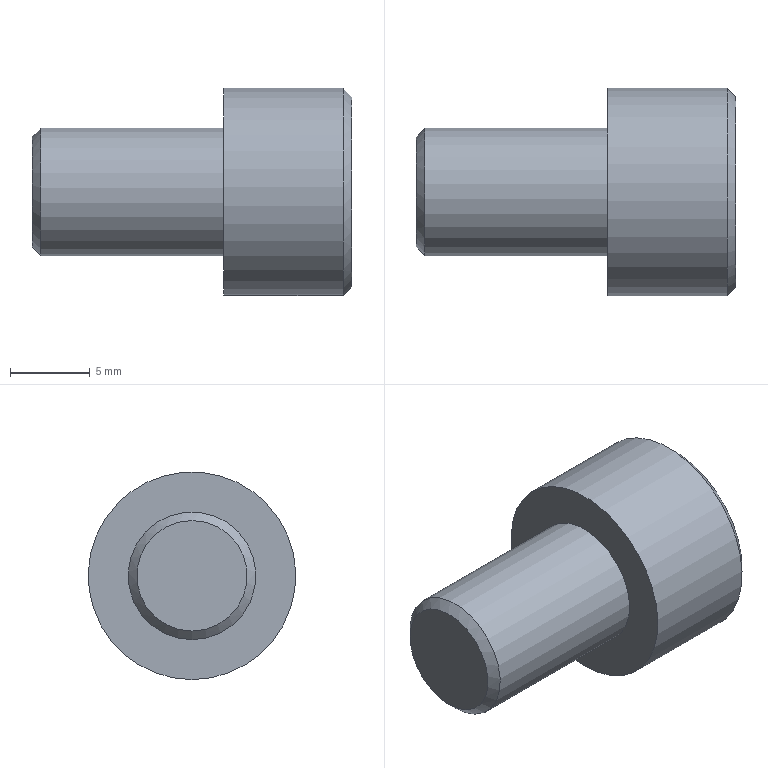Part | NX | features solid 2 | 1 solid | 7 faces | box 20 x 13 x 13 mm | volume 1656 mm3 | plane 3 | cylinder 2 | cone 2 | commonest cylinder face diameters 8 x1 13 x1
STEP:
#1=CARTESIAN_POINT('',(-160.54,1240.,-606.5));
#2=VERTEX_POINT('',#1);
#3=CARTESIAN_POINT('',(-160.54,1240.,-600.));
#4=DIRECTION('',(-1.,0.,0.));
#5=DIRECTION('',(0.,0.,-1.));
#6=AXIS2_PLACEMENT_3D('',#3,#4,#5);
#7=CIRCLE('',#6,6.5);
#8=EDGE_CURVE('',#2,#2,#7,.T.);
#9=ORIENTED_EDGE('',*,*,#8,.T.);
#10=EDGE_LOOP('',(#9));
#11=FACE_BOUND('',#10,.T.);
#12=CARTESIAN_POINT('',(-168.,1240.,-606.5));
#13=VERTEX_POINT('',#12);
#14=CARTESIAN_POINT('',(-168.,1240.,-600.));
#15=DIRECTION('',(-1.,0.,0.));
#16=DIRECTION('',(0.,0.,-1.));
#17=AXIS2_PLACEMENT_3D('',#14,#15,#16);
#18=CIRCLE('',#17,6.5);
#19=EDGE_CURVE('',#13,#13,#18,.T.);
#20=ORIENTED_EDGE('',*,*,#19,.F.);
#21=EDGE_LOOP('',(#20));
#22=FACE_BOUND('',#21,.T.);
#23=CARTESIAN_POINT('',(-168.,1240.,-600.));
#24=DIRECTION('',(1.,0.,0.));
#25=DIRECTION('',(0.,0.,1.));
#26=AXIS2_PLACEMENT_3D('',#23,#24,#25);
#27=CYLINDRICAL_SURFACE('',#26,6.5);
#28=ADVANCED_FACE('',(#11,#22),#27,.T.);
#29=CARTESIAN_POINT('',(-168.,1240.,-604.));
#30=VERTEX_POINT('',#29);
#31=CARTESIAN_POINT('',(-168.,1240.,-600.));
#32=DIRECTION('',(-1.,0.,0.));
#33=DIRECTION('',(0.,0.,-1.));
#34=AXIS2_PLACEMENT_3D('',#31,#32,#33);
#35=CIRCLE('',#34,4.);
#36=EDGE_CURVE('',#30,#30,#35,.T.);
#37=ORIENTED_EDGE('',*,*,#36,.F.);
#38=EDGE_LOOP('',(#37));
#39=FACE_BOUND('',#38,.T.);
#40=ORIENTED_EDGE('',*,*,#19,.T.);
#41=EDGE_LOOP('',(#40));
#42=FACE_BOUND('',#41,.T.);
#43=CARTESIAN_POINT('',(-168.,1240.,-600.));
#44=DIRECTION('',(-1.,0.,0.));
#45=DIRECTION('',(0.,0.,-1.));
#46=AXIS2_PLACEMENT_3D('',#43,#44,#45);
#47=PLANE('',#46);
#48=ADVANCED_FACE('',(#39,#42),#47,.T.);
#49=CARTESIAN_POINT('',(-160.,1240.,-605.96));
#50=VERTEX_POINT('',#49);
#51=CARTESIAN_POINT('',(-160.,1240.,-600.));
#52=DIRECTION('',(-1.,0.,0.));
#53=DIRECTION('',(0.,0.,-1.));
#54=AXIS2_PLACEMENT_3D('',#51,#52,#53);
#55=CIRCLE('',#54,5.96);
#56=EDGE_CURVE('',#50,#50,#55,.F.);
#57=ORIENTED_EDGE('',*,*,#56,.T.);
#58=EDGE_LOOP('',(#57));
#59=FACE_BOUND('',#58,.T.);
#60=CARTESIAN_POINT('',(-160.,1240.,-600.));
#61=DIRECTION('',(-1.,0.,0.));
#62=DIRECTION('',(0.,0.,-1.));
#63=AXIS2_PLACEMENT_3D('',#60,#61,#62);
#64=PLANE('',#63);
#65=ADVANCED_FACE('',(#59),#64,.F.);
#66=CARTESIAN_POINT('',(-179.46,1240.,-604.));
#67=VERTEX_POINT('',#66);
#68=CARTESIAN_POINT('',(-179.46,1240.,-600.));
#69=DIRECTION('',(-1.,0.,0.));
#70=DIRECTION('',(0.,0.,-1.));
#71=AXIS2_PLACEMENT_3D('',#68,#69,#70);
#72=CIRCLE('',#71,4.);
#73=EDGE_CURVE('',#67,#67,#72,.F.);
#74=ORIENTED_EDGE('',*,*,#73,.T.);
#75=EDGE_LOOP('',(#74));
#76=FACE_BOUND('',#75,.T.);
#77=ORIENTED_EDGE('',*,*,#36,.T.);
#78=EDGE_LOOP('',(#77));
#79=FACE_BOUND('',#78,.T.);
#80=CARTESIAN_POINT('',(-168.,1240.,-600.));
#81=DIRECTION('',(-1.,0.,0.));
#82=DIRECTION('',(0.,0.,-1.));
#83=AXIS2_PLACEMENT_3D('',#80,#81,#82);
#84=CYLINDRICAL_SURFACE('',#83,4.);
#85=ADVANCED_FACE('',(#76,#79),#84,.T.);
#86=CARTESIAN_POINT('',(-180.,1240.,-603.46));
#87=VERTEX_POINT('',#86);
#88=CARTESIAN_POINT('',(-180.,1240.,-600.));
#89=DIRECTION('',(-1.,0.,0.));
#90=DIRECTION('',(0.,0.,-1.));
#91=AXIS2_PLACEMENT_3D('',#88,#89,#90);
#92=CIRCLE('',#91,3.46);
#93=EDGE_CURVE('',#87,#87,#92,.T.);
#94=ORIENTED_EDGE('',*,*,#93,.T.);
#95=EDGE_LOOP('',(#94));
#96=FACE_BOUND('',#95,.T.);
#97=CARTESIAN_POINT('',(-180.,1240.,-600.));
#98=DIRECTION('',(-1.,0.,0.));
#99=DIRECTION('',(0.,0.,-1.));
#100=AXIS2_PLACEMENT_3D('',#97,#98,#99);
#101=PLANE('',#100);
#102=ADVANCED_FACE('',(#96),#101,.T.);
#103=ORIENTED_EDGE('',*,*,#73,.F.);
#104=EDGE_LOOP('',(#103));
#105=FACE_BOUND('',#104,.T.);
#106=ORIENTED_EDGE('',*,*,#93,.F.);
#107=EDGE_LOOP('',(#106));
#108=FACE_BOUND('',#107,.T.);
#109=CARTESIAN_POINT('',(-180.,1240.,-600.));
#110=DIRECTION('',(1.,0.,0.));
#111=DIRECTION('',(0.,0.,1.));
#112=AXIS2_PLACEMENT_3D('',#109,#110,#111);
#113=CONICAL_SURFACE('',#112,3.46,0.7854);
#114=ADVANCED_FACE('',(#105,#108),#113,.T.);
#115=ORIENTED_EDGE('',*,*,#56,.F.);
#116=EDGE_LOOP('',(#115));
#117=FACE_BOUND('',#116,.T.);
#118=ORIENTED_EDGE('',*,*,#8,.F.);
#119=EDGE_LOOP('',(#118));
#120=FACE_BOUND('',#119,.T.);
#121=CARTESIAN_POINT('',(-160.54,1240.,-600.));
#122=DIRECTION('',(-1.,0.,0.));
#123=DIRECTION('',(0.,0.,-1.));
#124=AXIS2_PLACEMENT_3D('',#121,#122,#123);
#125=CONICAL_SURFACE('',#124,6.5,0.7854);
#126=ADVANCED_FACE('',(#117,#120),#125,.T.);
#127=CLOSED_SHELL('',(#28,#48,#65,#85,#102,#114,#126));
#128=MANIFOLD_SOLID_BREP('',#127);
#129=(LENGTH_UNIT()NAMED_UNIT(*)SI_UNIT(.MILLI.,.METRE.));
#130=UNCERTAINTY_MEASURE_WITH_UNIT(LENGTH_MEASURE(0.00001),#129,'','');
#131=(NAMED_UNIT(*)PLANE_ANGLE_UNIT()SI_UNIT($,.RADIAN.));
#132=(NAMED_UNIT(*)SI_UNIT($,.STERADIAN.)SOLID_ANGLE_UNIT());
#133=(GEOMETRIC_REPRESENTATION_CONTEXT(3)GLOBAL_UNCERTAINTY_ASSIGNED_CONTEXT((#130))GLOBAL_UNIT_ASSIGNED_CONTEXT((#129,#131,#132))REPRESENTATION_CONTEXT('',''));
#134=ADVANCED_BREP_SHAPE_REPRESENTATION('',(#128),#133);